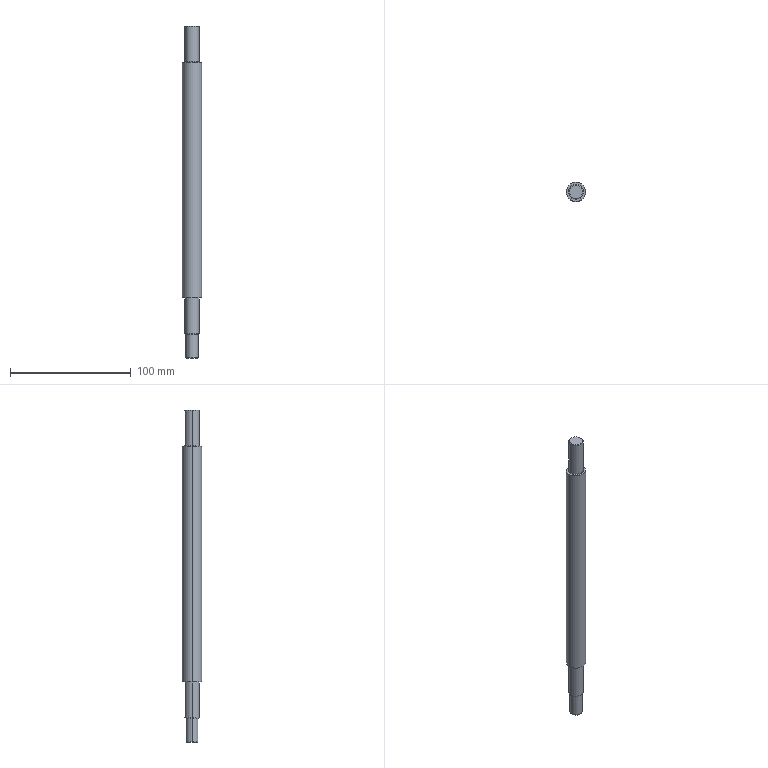Part | STEP file | 0230_001_MTSRK16-275-F30-R12-T30-Q12-S20-E10-BQ15 | 1 solid | 23 faces | box 16 x 16 x 275 mm | volume 47560 mm3 | cylinder 8 | torus 6 | plane 5 | cone 4 | commonest cylinder face diameters 12 x4 10 x2 16 x2
STEP:
#1=CARTESIAN_POINT('',(0.,0.,0.));
#2=DIRECTION('',(0.,0.,1.));
#3=DIRECTION('',(1.,0.,0.));
#4=AXIS2_PLACEMENT_3D('',#1,#2,#3);
#5=CARTESIAN_POINT('',(-4.6,0.,-245.));
#6=VERTEX_POINT('',#5);
#7=CARTESIAN_POINT('',(4.6,0.,-245.));
#8=VERTEX_POINT('',#7);
#9=CARTESIAN_POINT('',(0.,0.,-245.));
#10=DIRECTION('',(0.,0.,-1.));
#11=DIRECTION('',(-1.,0.,0.));
#12=AXIS2_PLACEMENT_3D('',#9,#10,#11);
#13=CIRCLE('',#12,4.6);
#14=CARTESIAN_POINT('',(0.,0.,-245.));
#15=DIRECTION('',(0.,0.,1.));
#16=DIRECTION('',(1.,0.,0.));
#17=AXIS2_PLACEMENT_3D('',#14,#15,#16);
#18=CONICAL_SURFACE('',#17,4.6,0.7854);
#19=CARTESIAN_POINT('',(3.142,0.));
#20=DIRECTION('',(-1.,0.));
#21=VECTOR('',#20,1.);
#22=LINE('',#19,#21);
#23=(GEOMETRIC_REPRESENTATION_CONTEXT(2)PARAMETRIC_REPRESENTATION_CONTEXT()REPRESENTATION_CONTEXT('',''));
#24=DEFINITIONAL_REPRESENTATION('',(#22),#23);
#25=PCURVE('',#18,#24);
#26=CARTESIAN_POINT('',(0.,0.,-245.));
#27=DIRECTION('',(0.,0.,-1.));
#28=DIRECTION('',(-1.,0.,0.));
#29=AXIS2_PLACEMENT_3D('',#26,#27,#28);
#30=PLANE('',#29);
#31=CARTESIAN_POINT('',(0.,0.));
#32=DIRECTION('',(1.,0.));
#33=AXIS2_PLACEMENT_2D('',#31,#32);
#34=CIRCLE('',#33,4.6);
#35=(GEOMETRIC_REPRESENTATION_CONTEXT(2)PARAMETRIC_REPRESENTATION_CONTEXT()REPRESENTATION_CONTEXT('',''));
#36=DEFINITIONAL_REPRESENTATION('',(#34),#35);
#37=PCURVE('',#30,#36);
#38=SURFACE_CURVE('',#13,(#25,#37),.PCURVE_S1.);
#39=EDGE_CURVE('',#6,#8,#38,.T.);
#40=ORIENTED_EDGE('',*,*,#39,.F.);
#41=CARTESIAN_POINT('',(-5.,0.,-244.6));
#42=VERTEX_POINT('',#41);
#43=CARTESIAN_POINT('',(-4.6,0.,-245.));
#44=DIRECTION('',(-0.7071,0.,0.7071));
#45=VECTOR('',#44,1.);
#46=LINE('',#43,#45);
#47=CARTESIAN_POINT('',(3.142,0.));
#48=DIRECTION('',(0.,1.));
#49=VECTOR('',#48,1.);
#50=LINE('',#47,#49);
#51=(GEOMETRIC_REPRESENTATION_CONTEXT(2)PARAMETRIC_REPRESENTATION_CONTEXT()REPRESENTATION_CONTEXT('',''));
#52=DEFINITIONAL_REPRESENTATION('',(#50),#51);
#53=PCURVE('',#18,#52);
#54=CARTESIAN_POINT('',(0.,0.,-245.));
#55=DIRECTION('',(0.,0.,1.));
#56=DIRECTION('',(1.,0.,0.));
#57=AXIS2_PLACEMENT_3D('',#54,#55,#56);
#58=CONICAL_SURFACE('',#57,4.6,0.7854);
#59=CARTESIAN_POINT('',(3.142,0.));
#60=DIRECTION('',(0.,1.));
#61=VECTOR('',#60,1.);
#62=LINE('',#59,#61);
#63=(GEOMETRIC_REPRESENTATION_CONTEXT(2)PARAMETRIC_REPRESENTATION_CONTEXT()REPRESENTATION_CONTEXT('',''));
#64=DEFINITIONAL_REPRESENTATION('',(#62),#63);
#65=PCURVE('',#58,#64);
#66=SURFACE_CURVE('',#46,(#53,#65),.PCURVE_S1.);
#67=EDGE_CURVE('',#6,#42,#66,.T.);
#68=ORIENTED_EDGE('',*,*,#67,.T.);
#69=CARTESIAN_POINT('',(5.,0.,-244.6));
#70=VERTEX_POINT('',#69);
#71=CARTESIAN_POINT('',(0.,0.,-244.6));
#72=DIRECTION('',(0.,0.,1.));
#73=DIRECTION('',(-1.,0.,0.));
#74=AXIS2_PLACEMENT_3D('',#71,#72,#73);
#75=CIRCLE('',#74,5.);
#76=CARTESIAN_POINT('',(-3.142,0.4));
#77=DIRECTION('',(1.,0.));
#78=VECTOR('',#77,1.);
#79=LINE('',#76,#78);
#80=(GEOMETRIC_REPRESENTATION_CONTEXT(2)PARAMETRIC_REPRESENTATION_CONTEXT()REPRESENTATION_CONTEXT('',''));
#81=DEFINITIONAL_REPRESENTATION('',(#79),#80);
#82=PCURVE('',#18,#81);
#83=CARTESIAN_POINT('',(0.,0.,30.));
#84=DIRECTION('',(0.,0.,-1.));
#85=DIRECTION('',(-1.,0.,0.));
#86=AXIS2_PLACEMENT_3D('',#83,#84,#85);
#87=CYLINDRICAL_SURFACE('',#86,5.);
#88=CARTESIAN_POINT('',(6.283,274.6));
#89=DIRECTION('',(-1.,0.));
#90=VECTOR('',#89,1.);
#91=LINE('',#88,#90);
#92=(GEOMETRIC_REPRESENTATION_CONTEXT(2)PARAMETRIC_REPRESENTATION_CONTEXT()REPRESENTATION_CONTEXT('',''));
#93=DEFINITIONAL_REPRESENTATION('',(#91),#92);
#94=PCURVE('',#87,#93);
#95=SURFACE_CURVE('',#75,(#82,#94),.PCURVE_S1.);
#96=EDGE_CURVE('',#70,#42,#95,.T.);
#97=ORIENTED_EDGE('',*,*,#96,.F.);
#98=CARTESIAN_POINT('',(4.6,0.,-245.));
#99=DIRECTION('',(0.7071,0.,0.7071));
#100=VECTOR('',#99,1.);
#101=LINE('',#98,#100);
#102=CARTESIAN_POINT('',(0.,0.));
#103=DIRECTION('',(0.,1.));
#104=VECTOR('',#103,1.);
#105=LINE('',#102,#104);
#106=(GEOMETRIC_REPRESENTATION_CONTEXT(2)PARAMETRIC_REPRESENTATION_CONTEXT()REPRESENTATION_CONTEXT('',''));
#107=DEFINITIONAL_REPRESENTATION('',(#105),#106);
#108=PCURVE('',#18,#107);
#109=CARTESIAN_POINT('',(6.283,0.));
#110=DIRECTION('',(0.,1.));
#111=VECTOR('',#110,1.);
#112=LINE('',#109,#111);
#113=(GEOMETRIC_REPRESENTATION_CONTEXT(2)PARAMETRIC_REPRESENTATION_CONTEXT()REPRESENTATION_CONTEXT('',''));
#114=DEFINITIONAL_REPRESENTATION('',(#112),#113);
#115=PCURVE('',#58,#114);
#116=SURFACE_CURVE('',#101,(#108,#115),.PCURVE_S1.);
#117=EDGE_CURVE('',#8,#70,#116,.T.);
#118=ORIENTED_EDGE('',*,*,#117,.F.);
#119=EDGE_LOOP('',(#40,#68,#97,#118));
#120=FACE_BOUND('',#119,.T.);
#121=ADVANCED_FACE('',(#120),#18,.T.);
#122=CARTESIAN_POINT('',(5.6,0.,30.));
#123=VERTEX_POINT('',#122);
#124=CARTESIAN_POINT('',(-5.6,0.,30.));
#125=VERTEX_POINT('',#124);
#126=CARTESIAN_POINT('',(0.,0.,30.));
#127=DIRECTION('',(0.,0.,1.));
#128=DIRECTION('',(1.,0.,0.));
#129=AXIS2_PLACEMENT_3D('',#126,#127,#128);
#130=CIRCLE('',#129,5.6);
#131=CARTESIAN_POINT('',(0.,0.,29.6));
#132=DIRECTION('',(0.,0.,-1.));
#133=DIRECTION('',(-1.,0.,0.));
#134=AXIS2_PLACEMENT_3D('',#131,#132,#133);
#135=CONICAL_SURFACE('',#134,6.,0.7854);
#136=CARTESIAN_POINT('',(3.142,-0.4));
#137=DIRECTION('',(-1.,0.));
#138=VECTOR('',#137,1.);
#139=LINE('',#136,#138);
#140=(GEOMETRIC_REPRESENTATION_CONTEXT(2)PARAMETRIC_REPRESENTATION_CONTEXT()REPRESENTATION_CONTEXT('',''));
#141=DEFINITIONAL_REPRESENTATION('',(#139),#140);
#142=PCURVE('',#135,#141);
#143=CARTESIAN_POINT('',(6.,0.,30.));
#144=DIRECTION('',(0.,0.,1.));
#145=DIRECTION('',(1.,0.,0.));
#146=AXIS2_PLACEMENT_3D('',#143,#144,#145);
#147=PLANE('',#146);
#148=CARTESIAN_POINT('',(-6.,0.));
#149=DIRECTION('',(1.,0.));
#150=AXIS2_PLACEMENT_2D('',#148,#149);
#151=CIRCLE('',#150,5.6);
#152=(GEOMETRIC_REPRESENTATION_CONTEXT(2)PARAMETRIC_REPRESENTATION_CONTEXT()REPRESENTATION_CONTEXT('',''));
#153=DEFINITIONAL_REPRESENTATION('',(#151),#152);
#154=PCURVE('',#147,#153);
#155=SURFACE_CURVE('',#130,(#142,#154),.PCURVE_S1.);
#156=EDGE_CURVE('',#123,#125,#155,.T.);
#157=ORIENTED_EDGE('',*,*,#156,.F.);
#158=CARTESIAN_POINT('',(6.,0.,29.6));
#159=VERTEX_POINT('',#158);
#160=CARTESIAN_POINT('',(6.,0.,29.6));
#161=DIRECTION('',(0.7071,0.,-0.7071));
#162=VECTOR('',#161,1.);
#163=LINE('',#160,#162);
#164=CARTESIAN_POINT('',(3.142,0.));
#165=DIRECTION('',(0.,1.));
#166=VECTOR('',#165,1.);
#167=LINE('',#164,#166);
#168=(GEOMETRIC_REPRESENTATION_CONTEXT(2)PARAMETRIC_REPRESENTATION_CONTEXT()REPRESENTATION_CONTEXT('',''));
#169=DEFINITIONAL_REPRESENTATION('',(#167),#168);
#170=PCURVE('',#135,#169);
#171=CARTESIAN_POINT('',(0.,0.,29.6));
#172=DIRECTION('',(0.,0.,-1.));
#173=DIRECTION('',(-1.,0.,0.));
#174=AXIS2_PLACEMENT_3D('',#171,#172,#173);
#175=CONICAL_SURFACE('',#174,6.,0.7854);
#176=CARTESIAN_POINT('',(3.142,0.));
#177=DIRECTION('',(0.,1.));
#178=VECTOR('',#177,1.);
#179=LINE('',#176,#178);
#180=(GEOMETRIC_REPRESENTATION_CONTEXT(2)PARAMETRIC_REPRESENTATION_CONTEXT()REPRESENTATION_CONTEXT('',''));
#181=DEFINITIONAL_REPRESENTATION('',(#179),#180);
#182=PCURVE('',#175,#181);
#183=SURFACE_CURVE('',#163,(#170,#182),.PCURVE_S1.);
#184=EDGE_CURVE('',#123,#159,#183,.T.);
#185=ORIENTED_EDGE('',*,*,#184,.T.);
#186=CARTESIAN_POINT('',(-6.,0.,29.6));
#187=VERTEX_POINT('',#186);
#188=CARTESIAN_POINT('',(0.,0.,29.6));
#189=DIRECTION('',(0.,0.,-1.));
#190=DIRECTION('',(1.,0.,0.));
#191=AXIS2_PLACEMENT_3D('',#188,#189,#190);
#192=CIRCLE('',#191,6.);
#193=CARTESIAN_POINT('',(-3.142,0.));
#194=DIRECTION('',(1.,0.));
#195=VECTOR('',#194,1.);
#196=LINE('',#193,#195);
#197=(GEOMETRIC_REPRESENTATION_CONTEXT(2)PARAMETRIC_REPRESENTATION_CONTEXT()REPRESENTATION_CONTEXT('',''));
#198=DEFINITIONAL_REPRESENTATION('',(#196),#197);
#199=PCURVE('',#135,#198);
#200=CARTESIAN_POINT('',(0.,0.,30.));
#201=DIRECTION('',(0.,0.,-1.));
#202=DIRECTION('',(-1.,0.,0.));
#203=AXIS2_PLACEMENT_3D('',#200,#201,#202);
#204=CYLINDRICAL_SURFACE('',#203,6.);
#205=CARTESIAN_POINT('',(-3.142,0.4));
#206=DIRECTION('',(1.,0.));
#207=VECTOR('',#206,1.);
#208=LINE('',#205,#207);
#209=(GEOMETRIC_REPRESENTATION_CONTEXT(2)PARAMETRIC_REPRESENTATION_CONTEXT()REPRESENTATION_CONTEXT('',''));
#210=DEFINITIONAL_REPRESENTATION('',(#208),#209);
#211=PCURVE('',#204,#210);
#212=SURFACE_CURVE('',#192,(#199,#211),.PCURVE_S1.);
#213=EDGE_CURVE('',#187,#159,#212,.T.);
#214=ORIENTED_EDGE('',*,*,#213,.F.);
#215=CARTESIAN_POINT('',(-6.,0.,29.6));
#216=DIRECTION('',(-0.7071,0.,-0.7071));
#217=VECTOR('',#216,1.);
#218=LINE('',#215,#217);
#219=CARTESIAN_POINT('',(0.,0.));
#220=DIRECTION('',(0.,1.));
#221=VECTOR('',#220,1.);
#222=LINE('',#219,#221);
#223=(GEOMETRIC_REPRESENTATION_CONTEXT(2)PARAMETRIC_REPRESENTATION_CONTEXT()REPRESENTATION_CONTEXT('',''));
#224=DEFINITIONAL_REPRESENTATION('',(#222),#223);
#225=PCURVE('',#135,#224);
#226=CARTESIAN_POINT('',(6.283,0.));
#227=DIRECTION('',(0.,1.));
#228=VECTOR('',#227,1.);
#229=LINE('',#226,#228);
#230=(GEOMETRIC_REPRESENTATION_CONTEXT(2)PARAMETRIC_REPRESENTATION_CONTEXT()REPRESENTATION_CONTEXT('',''));
#231=DEFINITIONAL_REPRESENTATION('',(#229),#230);
#232=PCURVE('',#175,#231);
#233=SURFACE_CURVE('',#218,(#225,#232),.PCURVE_S1.);
#234=EDGE_CURVE('',#125,#187,#233,.T.);
#235=ORIENTED_EDGE('',*,*,#234,.F.);
#236=EDGE_LOOP('',(#157,#185,#214,#235));
#237=FACE_BOUND('',#236,.T.);
#238=ADVANCED_FACE('',(#237),#135,.T.);
#239=CARTESIAN_POINT('',(6.,0.,0.3));
#240=VERTEX_POINT('',#239);
#241=CARTESIAN_POINT('',(6.3,0.,0.));
#242=VERTEX_POINT('',#241);
#243=CARTESIAN_POINT('',(6.3,0.,0.3));
#244=DIRECTION('',(0.,-1.,0.));
#245=DIRECTION('',(0.,0.,-1.));
#246=AXIS2_PLACEMENT_3D('',#243,#244,#245);
#247=CIRCLE('',#246,0.3);
#248=CARTESIAN_POINT('',(0.,0.,0.3));
#249=DIRECTION('',(0.,0.,1.));
#250=DIRECTION('',(1.,0.,0.));
#251=AXIS2_PLACEMENT_3D('',#248,#249,#250);
#252=TOROIDAL_SURFACE('',#251,6.3,0.3);
#253=CARTESIAN_POINT('',(6.283,-1.571));
#254=DIRECTION('',(0.,1.));
#255=VECTOR('',#254,1.);
#256=LINE('',#253,#255);
#257=(GEOMETRIC_REPRESENTATION_CONTEXT(2)PARAMETRIC_REPRESENTATION_CONTEXT()REPRESENTATION_CONTEXT('',''));
#258=DEFINITIONAL_REPRESENTATION('',(#256),#257);
#259=PCURVE('',#252,#258);
#260=CARTESIAN_POINT('',(0.,0.,0.3));
#261=DIRECTION('',(0.,0.,1.));
#262=DIRECTION('',(1.,0.,0.));
#263=AXIS2_PLACEMENT_3D('',#260,#261,#262);
#264=TOROIDAL_SURFACE('',#263,6.3,0.3);
#265=CARTESIAN_POINT('',(0.,-1.571));
#266=DIRECTION('',(0.,1.));
#267=VECTOR('',#266,1.);
#268=LINE('',#265,#267);
#269=(GEOMETRIC_REPRESENTATION_CONTEXT(2)PARAMETRIC_REPRESENTATION_CONTEXT()REPRESENTATION_CONTEXT('',''));
#270=DEFINITIONAL_REPRESENTATION('',(#268),#269);
#271=PCURVE('',#264,#270);
#272=SURFACE_CURVE('',#247,(#259,#271),.PCURVE_S1.);
#273=EDGE_CURVE('',#240,#242,#272,.T.);
#274=ORIENTED_EDGE('',*,*,#273,.T.);
#275=CARTESIAN_POINT('',(-6.3,0.,0.));
#276=VERTEX_POINT('',#275);
#277=CARTESIAN_POINT('',(0.,0.,0.));
#278=DIRECTION('',(0.,0.,-1.));
#279=DIRECTION('',(1.,0.,0.));
#280=AXIS2_PLACEMENT_3D('',#277,#278,#279);
#281=CIRCLE('',#280,6.3);
#282=CARTESIAN_POINT('',(6.283,4.712));
#283=DIRECTION('',(-1.,0.));
#284=VECTOR('',#283,1.);
#285=LINE('',#282,#284);
#286=(GEOMETRIC_REPRESENTATION_CONTEXT(2)PARAMETRIC_REPRESENTATION_CONTEXT()REPRESENTATION_CONTEXT('',''));
#287=DEFINITIONAL_REPRESENTATION('',(#285),#286);
#288=PCURVE('',#252,#287);
#289=CARTESIAN_POINT('',(8.,0.,0.));
#290=DIRECTION('',(0.,0.,1.));
#291=DIRECTION('',(1.,0.,0.));
#292=AXIS2_PLACEMENT_3D('',#289,#290,#291);
#293=PLANE('',#292);
#294=CARTESIAN_POINT('',(-1.7,0.));
#295=CARTESIAN_POINT('',(-1.7,-10.912));
#296=CARTESIAN_POINT('',(-11.15,-5.456));
#297=CARTESIAN_POINT('',(-20.6,0.));
#298=CARTESIAN_POINT('',(-11.15,5.456));
#299=CARTESIAN_POINT('',(-1.7,10.912));
#300=CARTESIAN_POINT('',(-1.7,0.));
#301=(BOUNDED_CURVE()B_SPLINE_CURVE(2,(#294,#295,#296,#297,#298,#299,#300),.UNSPECIFIED.,.T.,.F.)B_SPLINE_CURVE_WITH_KNOTS((1,2,2,2,2,1),(-2.094,0.,2.094,4.189,6.283,8.378),.UNSPECIFIED.)CURVE()GEOMETRIC_REPRESENTATION_ITEM()RATIONAL_B_SPLINE_CURVE((1.,0.5,1.,0.5,1.,0.5,1.))REPRESENTATION_ITEM(''));
#302=(GEOMETRIC_REPRESENTATION_CONTEXT(2)PARAMETRIC_REPRESENTATION_CONTEXT()REPRESENTATION_CONTEXT('',''));
#303=DEFINITIONAL_REPRESENTATION('',(#301),#302);
#304=PCURVE('',#293,#303);
#305=SURFACE_CURVE('',#281,(#288,#304),.PCURVE_S1.);
#306=EDGE_CURVE('',#242,#276,#305,.T.);
#307=ORIENTED_EDGE('',*,*,#306,.T.);
#308=CARTESIAN_POINT('',(-6.,0.,0.3));
#309=VERTEX_POINT('',#308);
#310=CARTESIAN_POINT('',(-6.3,0.,0.3));
#311=DIRECTION('',(0.,1.,0.));
#312=DIRECTION('',(-1.,0.,0.));
#313=AXIS2_PLACEMENT_3D('',#310,#311,#312);
#314=CIRCLE('',#313,0.3);
#315=CARTESIAN_POINT('',(3.142,0.));
#316=DIRECTION('',(0.,1.));
#317=VECTOR('',#316,1.);
#318=LINE('',#315,#317);
#319=(GEOMETRIC_REPRESENTATION_CONTEXT(2)PARAMETRIC_REPRESENTATION_CONTEXT()REPRESENTATION_CONTEXT('',''));
#320=DEFINITIONAL_REPRESENTATION('',(#318),#319);
#321=PCURVE('',#252,#320);
#322=CARTESIAN_POINT('',(3.142,0.));
#323=DIRECTION('',(0.,1.));
#324=VECTOR('',#323,1.);
#325=LINE('',#322,#324);
#326=(GEOMETRIC_REPRESENTATION_CONTEXT(2)PARAMETRIC_REPRESENTATION_CONTEXT()REPRESENTATION_CONTEXT('',''));
#327=DEFINITIONAL_REPRESENTATION('',(#325),#326);
#328=PCURVE('',#264,#327);
#329=SURFACE_CURVE('',#314,(#321,#328),.PCURVE_S1.);
#330=EDGE_CURVE('',#309,#276,#329,.T.);
#331=ORIENTED_EDGE('',*,*,#330,.F.);
#332=CARTESIAN_POINT('',(0.,0.,0.3));
#333=DIRECTION('',(0.,0.,1.));
#334=DIRECTION('',(1.,0.,0.));
#335=AXIS2_PLACEMENT_3D('',#332,#333,#334);
#336=CIRCLE('',#335,6.);
#337=CARTESIAN_POINT('',(0.,3.142));
#338=DIRECTION('',(1.,0.));
#339=VECTOR('',#338,1.);
#340=LINE('',#337,#339);
#341=(GEOMETRIC_REPRESENTATION_CONTEXT(2)PARAMETRIC_REPRESENTATION_CONTEXT()REPRESENTATION_CONTEXT('',''));
#342=DEFINITIONAL_REPRESENTATION('',(#340),#341);
#343=PCURVE('',#252,#342);
#344=CARTESIAN_POINT('',(0.,0.,30.));
#345=DIRECTION('',(0.,0.,-1.));
#346=DIRECTION('',(-1.,0.,0.));
#347=AXIS2_PLACEMENT_3D('',#344,#345,#346);
#348=CYLINDRICAL_SURFACE('',#347,6.);
#349=CARTESIAN_POINT('',(9.425,29.7));
#350=DIRECTION('',(-1.,0.));
#351=VECTOR('',#350,1.);
#352=LINE('',#349,#351);
#353=(GEOMETRIC_REPRESENTATION_CONTEXT(2)PARAMETRIC_REPRESENTATION_CONTEXT()REPRESENTATION_CONTEXT('',''));
#354=DEFINITIONAL_REPRESENTATION('',(#352),#353);
#355=PCURVE('',#348,#354);
#356=SURFACE_CURVE('',#336,(#343,#355),.PCURVE_S1.);
#357=EDGE_CURVE('',#309,#240,#356,.T.);
#358=ORIENTED_EDGE('',*,*,#357,.T.);
#359=EDGE_LOOP('',(#274,#307,#331,#358));
#360=FACE_BOUND('',#359,.F.);
#361=ADVANCED_FACE('',(#360),#252,.F.);
#362=CARTESIAN_POINT('',(-6.,0.,-195.3));
#363=VERTEX_POINT('',#362);
#364=CARTESIAN_POINT('',(-6.3,0.,-195.));
#365=VERTEX_POINT('',#364);
#366=CARTESIAN_POINT('',(-6.3,0.,-195.3));
#367=DIRECTION('',(0.,-1.,0.));
#368=DIRECTION('',(0.,0.,-1.));
#369=AXIS2_PLACEMENT_3D('',#366,#367,#368);
#370=CIRCLE('',#369,0.3);
#371=CARTESIAN_POINT('',(0.,0.,-195.3));
#372=DIRECTION('',(0.,0.,-1.));
#373=DIRECTION('',(-1.,0.,0.));
#374=AXIS2_PLACEMENT_3D('',#371,#372,#373);
#375=TOROIDAL_SURFACE('',#374,6.3,0.3);
#376=CARTESIAN_POINT('',(6.283,1.571));
#377=DIRECTION('',(0.,1.));
#378=VECTOR('',#377,1.);
#379=LINE('',#376,#378);
#380=(GEOMETRIC_REPRESENTATION_CONTEXT(2)PARAMETRIC_REPRESENTATION_CONTEXT()REPRESENTATION_CONTEXT('',''));
#381=DEFINITIONAL_REPRESENTATION('',(#379),#380);
#382=PCURVE('',#375,#381);
#383=CARTESIAN_POINT('',(0.,0.,-195.3));
#384=DIRECTION('',(0.,0.,-1.));
#385=DIRECTION('',(-1.,0.,0.));
#386=AXIS2_PLACEMENT_3D('',#383,#384,#385);
#387=TOROIDAL_SURFACE('',#386,6.3,0.3);
#388=CARTESIAN_POINT('',(0.,1.571));
#389=DIRECTION('',(0.,1.));
#390=VECTOR('',#389,1.);
#391=LINE('',#388,#390);
#392=(GEOMETRIC_REPRESENTATION_CONTEXT(2)PARAMETRIC_REPRESENTATION_CONTEXT()REPRESENTATION_CONTEXT('',''));
#393=DEFINITIONAL_REPRESENTATION('',(#391),#392);
#394=PCURVE('',#387,#393);
#395=SURFACE_CURVE('',#370,(#382,#394),.PCURVE_S1.);
#396=EDGE_CURVE('',#363,#365,#395,.T.);
#397=ORIENTED_EDGE('',*,*,#396,.T.);
#398=CARTESIAN_POINT('',(6.3,0.,-195.));
#399=VERTEX_POINT('',#398);
#400=CARTESIAN_POINT('',(0.,0.,-195.));
#401=DIRECTION('',(0.,0.,1.));
#402=DIRECTION('',(-1.,0.,0.));
#403=AXIS2_PLACEMENT_3D('',#400,#401,#402);
#404=CIRCLE('',#403,6.3);
#405=CARTESIAN_POINT('',(6.283,4.712));
#406=DIRECTION('',(-1.,0.));
#407=VECTOR('',#406,1.);
#408=LINE('',#405,#407);
#409=(GEOMETRIC_REPRESENTATION_CONTEXT(2)PARAMETRIC_REPRESENTATION_CONTEXT()REPRESENTATION_CONTEXT('',''));
#410=DEFINITIONAL_REPRESENTATION('',(#408),#409);
#411=PCURVE('',#375,#410);
#412=CARTESIAN_POINT('',(6.,0.,-195.));
#413=DIRECTION('',(0.,0.,-1.));
#414=DIRECTION('',(-1.,0.,0.));
#415=AXIS2_PLACEMENT_3D('',#412,#413,#414);
#416=PLANE('',#415);
#417=CARTESIAN_POINT('',(12.3,0.));
#418=CARTESIAN_POINT('',(12.3,-10.912));
#419=CARTESIAN_POINT('',(2.85,-5.456));
#420=CARTESIAN_POINT('',(-6.6,0.));
#421=CARTESIAN_POINT('',(2.85,5.456));
#422=CARTESIAN_POINT('',(12.3,10.912));
#423=CARTESIAN_POINT('',(12.3,0.));
#424=(BOUNDED_CURVE()B_SPLINE_CURVE(2,(#417,#418,#419,#420,#421,#422,#423),.UNSPECIFIED.,.T.,.F.)B_SPLINE_CURVE_WITH_KNOTS((1,2,2,2,2,1),(-2.094,0.,2.094,4.189,6.283,8.378),.UNSPECIFIED.)CURVE()GEOMETRIC_REPRESENTATION_ITEM()RATIONAL_B_SPLINE_CURVE((1.,0.5,1.,0.5,1.,0.5,1.))REPRESENTATION_ITEM(''));
#425=(GEOMETRIC_REPRESENTATION_CONTEXT(2)PARAMETRIC_REPRESENTATION_CONTEXT()REPRESENTATION_CONTEXT('',''));
#426=DEFINITIONAL_REPRESENTATION('',(#424),#425);
#427=PCURVE('',#416,#426);
#428=SURFACE_CURVE('',#404,(#411,#427),.PCURVE_S1.);
#429=EDGE_CURVE('',#365,#399,#428,.T.);
#430=ORIENTED_EDGE('',*,*,#429,.T.);
#431=CARTESIAN_POINT('',(6.,0.,-195.3));
#432=VERTEX_POINT('',#431);
#433=CARTESIAN_POINT('',(6.3,0.,-195.3));
#434=DIRECTION('',(0.,1.,0.));
#435=DIRECTION('',(-1.,0.,0.));
#436=AXIS2_PLACEMENT_3D('',#433,#434,#435);
#437=CIRCLE('',#436,0.3);
#438=CARTESIAN_POINT('',(3.142,3.142));
#439=DIRECTION('',(0.,1.));
#440=VECTOR('',#439,1.);
#441=LINE('',#438,#440);
#442=(GEOMETRIC_REPRESENTATION_CONTEXT(2)PARAMETRIC_REPRESENTATION_CONTEXT()REPRESENTATION_CONTEXT('',''));
#443=DEFINITIONAL_REPRESENTATION('',(#441),#442);
#444=PCURVE('',#375,#443);
#445=CARTESIAN_POINT('',(3.142,3.142));
#446=DIRECTION('',(0.,1.));
#447=VECTOR('',#446,1.);
#448=LINE('',#445,#447);
#449=(GEOMETRIC_REPRESENTATION_CONTEXT(2)PARAMETRIC_REPRESENTATION_CONTEXT()REPRESENTATION_CONTEXT('',''));
#450=DEFINITIONAL_REPRESENTATION('',(#448),#449);
#451=PCURVE('',#387,#450);
#452=SURFACE_CURVE('',#437,(#444,#451),.PCURVE_S1.);
#453=EDGE_CURVE('',#432,#399,#452,.T.);
#454=ORIENTED_EDGE('',*,*,#453,.F.);
#455=CARTESIAN_POINT('',(0.,0.,-195.3));
#456=DIRECTION('',(0.,0.,-1.));
#457=DIRECTION('',(-1.,0.,0.));
#458=AXIS2_PLACEMENT_3D('',#455,#456,#457);
#459=CIRCLE('',#458,6.);
#460=CARTESIAN_POINT('',(0.,3.142));
#461=DIRECTION('',(1.,0.));
#462=VECTOR('',#461,1.);
#463=LINE('',#460,#462);
#464=(GEOMETRIC_REPRESENTATION_CONTEXT(2)PARAMETRIC_REPRESENTATION_CONTEXT()REPRESENTATION_CONTEXT('',''));
#465=DEFINITIONAL_REPRESENTATION('',(#463),#464);
#466=PCURVE('',#375,#465);
#467=CARTESIAN_POINT('',(0.,0.,30.));
#468=DIRECTION('',(0.,0.,-1.));
#469=DIRECTION('',(-1.,0.,0.));
#470=AXIS2_PLACEMENT_3D('',#467,#468,#469);
#471=CYLINDRICAL_SURFACE('',#470,6.);
#472=CARTESIAN_POINT('',(0.,225.3));
#473=DIRECTION('',(1.,0.));
#474=VECTOR('',#473,1.);
#475=LINE('',#472,#474);
#476=(GEOMETRIC_REPRESENTATION_CONTEXT(2)PARAMETRIC_REPRESENTATION_CONTEXT()REPRESENTATION_CONTEXT('',''));
#477=DEFINITIONAL_REPRESENTATION('',(#475),#476);
#478=PCURVE('',#471,#477);
#479=SURFACE_CURVE('',#459,(#466,#478),.PCURVE_S1.);
#480=EDGE_CURVE('',#432,#363,#479,.T.);
#481=ORIENTED_EDGE('',*,*,#480,.T.);
#482=EDGE_LOOP('',(#397,#430,#454,#481));
#483=FACE_BOUND('',#482,.F.);
#484=ADVANCED_FACE('',(#483),#375,.F.);
#485=CARTESIAN_POINT('',(-5.,0.,-225.3));
#486=VERTEX_POINT('',#485);
#487=CARTESIAN_POINT('',(-5.3,0.,-225.));
#488=VERTEX_POINT('',#487);
#489=CARTESIAN_POINT('',(-5.3,0.,-225.3));
#490=DIRECTION('',(0.,-1.,0.));
#491=DIRECTION('',(0.,0.,-1.));
#492=AXIS2_PLACEMENT_3D('',#489,#490,#491);
#493=CIRCLE('',#492,0.3);
#494=CARTESIAN_POINT('',(0.,0.,-225.3));
#495=DIRECTION('',(0.,0.,-1.));
#496=DIRECTION('',(-1.,0.,0.));
#497=AXIS2_PLACEMENT_3D('',#494,#495,#496);
#498=TOROIDAL_SURFACE('',#497,5.3,0.3);
#499=CARTESIAN_POINT('',(6.283,1.571));
#500=DIRECTION('',(0.,1.));
#501=VECTOR('',#500,1.);
#502=LINE('',#499,#501);
#503=(GEOMETRIC_REPRESENTATION_CONTEXT(2)PARAMETRIC_REPRESENTATION_CONTEXT()REPRESENTATION_CONTEXT('',''));
#504=DEFINITIONAL_REPRESENTATION('',(#502),#503);
#505=PCURVE('',#498,#504);
#506=CARTESIAN_POINT('',(0.,0.,-225.3));
#507=DIRECTION('',(0.,0.,-1.));
#508=DIRECTION('',(-1.,0.,0.));
#509=AXIS2_PLACEMENT_3D('',#506,#507,#508);
#510=TOROIDAL_SURFACE('',#509,5.3,0.3);
#511=CARTESIAN_POINT('',(0.,1.571));
#512=DIRECTION('',(0.,1.));
#513=VECTOR('',#512,1.);
#514=LINE('',#511,#513);
#515=(GEOMETRIC_REPRESENTATION_CONTEXT(2)PARAMETRIC_REPRESENTATION_CONTEXT()REPRESENTATION_CONTEXT('',''));
#516=DEFINITIONAL_REPRESENTATION('',(#514),#515);
#517=PCURVE('',#510,#516);
#518=SURFACE_CURVE('',#493,(#505,#517),.PCURVE_S1.);
#519=EDGE_CURVE('',#486,#488,#518,.T.);
#520=ORIENTED_EDGE('',*,*,#519,.T.);
#521=CARTESIAN_POINT('',(5.3,0.,-225.));
#522=VERTEX_POINT('',#521);
#523=CARTESIAN_POINT('',(0.,0.,-225.));
#524=DIRECTION('',(0.,0.,1.));
#525=DIRECTION('',(-1.,0.,0.));
#526=AXIS2_PLACEMENT_3D('',#523,#524,#525);
#527=CIRCLE('',#526,5.3);
#528=CARTESIAN_POINT('',(6.283,4.712));
#529=DIRECTION('',(-1.,0.));
#530=VECTOR('',#529,1.);
#531=LINE('',#528,#530);
#532=(GEOMETRIC_REPRESENTATION_CONTEXT(2)PARAMETRIC_REPRESENTATION_CONTEXT()REPRESENTATION_CONTEXT('',''));
#533=DEFINITIONAL_REPRESENTATION('',(#531),#532);
#534=PCURVE('',#498,#533);
#535=CARTESIAN_POINT('',(5.,0.,-225.));
#536=DIRECTION('',(0.,0.,-1.));
#537=DIRECTION('',(-1.,0.,0.));
#538=AXIS2_PLACEMENT_3D('',#535,#536,#537);
#539=PLANE('',#538);
#540=CARTESIAN_POINT('',(10.3,0.));
#541=CARTESIAN_POINT('',(10.3,-9.18));
#542=CARTESIAN_POINT('',(2.35,-4.59));
#543=CARTESIAN_POINT('',(-5.6,0.));
#544=CARTESIAN_POINT('',(2.35,4.59));
#545=CARTESIAN_POINT('',(10.3,9.18));
#546=CARTESIAN_POINT('',(10.3,0.));
#547=(BOUNDED_CURVE()B_SPLINE_CURVE(2,(#540,#541,#542,#543,#544,#545,#546),.UNSPECIFIED.,.T.,.F.)B_SPLINE_CURVE_WITH_KNOTS((1,2,2,2,2,1),(-2.094,0.,2.094,4.189,6.283,8.378),.UNSPECIFIED.)CURVE()GEOMETRIC_REPRESENTATION_ITEM()RATIONAL_B_SPLINE_CURVE((1.,0.5,1.,0.5,1.,0.5,1.))REPRESENTATION_ITEM(''));
#548=(GEOMETRIC_REPRESENTATION_CONTEXT(2)PARAMETRIC_REPRESENTATION_CONTEXT()REPRESENTATION_CONTEXT('',''));
#549=DEFINITIONAL_REPRESENTATION('',(#547),#548);
#550=PCURVE('',#539,#549);
#551=SURFACE_CURVE('',#527,(#534,#550),.PCURVE_S1.);
#552=EDGE_CURVE('',#488,#522,#551,.T.);
#553=ORIENTED_EDGE('',*,*,#552,.T.);
#554=CARTESIAN_POINT('',(5.,0.,-225.3));
#555=VERTEX_POINT('',#554);
#556=CARTESIAN_POINT('',(5.3,0.,-225.3));
#557=DIRECTION('',(0.,1.,0.));
#558=DIRECTION('',(-1.,0.,0.));
#559=AXIS2_PLACEMENT_3D('',#556,#557,#558);
#560=CIRCLE('',#559,0.3);
#561=CARTESIAN_POINT('',(3.142,3.142));
#562=DIRECTION('',(0.,1.));
#563=VECTOR('',#562,1.);
#564=LINE('',#561,#563);
#565=(GEOMETRIC_REPRESENTATION_CONTEXT(2)PARAMETRIC_REPRESENTATION_CONTEXT()REPRESENTATION_CONTEXT('',''));
#566=DEFINITIONAL_REPRESENTATION('',(#564),#565);
#567=PCURVE('',#498,#566);
#568=CARTESIAN_POINT('',(3.142,3.142));
#569=DIRECTION('',(0.,1.));
#570=VECTOR('',#569,1.);
#571=LINE('',#568,#570);
#572=(GEOMETRIC_REPRESENTATION_CONTEXT(2)PARAMETRIC_REPRESENTATION_CONTEXT()REPRESENTATION_CONTEXT('',''));
#573=DEFINITIONAL_REPRESENTATION('',(#571),#572);
#574=PCURVE('',#510,#573);
#575=SURFACE_CURVE('',#560,(#567,#574),.PCURVE_S1.);
#576=EDGE_CURVE('',#555,#522,#575,.T.);
#577=ORIENTED_EDGE('',*,*,#576,.F.);
#578=CARTESIAN_POINT('',(0.,0.,-225.3));
#579=DIRECTION('',(0.,0.,-1.));
#580=DIRECTION('',(-1.,0.,0.));
#581=AXIS2_PLACEMENT_3D('',#578,#579,#580);
#582=CIRCLE('',#581,5.);
#583=CARTESIAN_POINT('',(0.,3.142));
#584=DIRECTION('',(1.,0.));
#585=VECTOR('',#584,1.);
#586=LINE('',#583,#585);
#587=(GEOMETRIC_REPRESENTATION_CONTEXT(2)PARAMETRIC_REPRESENTATION_CONTEXT()REPRESENTATION_CONTEXT('',''));
#588=DEFINITIONAL_REPRESENTATION('',(#586),#587);
#589=PCURVE('',#498,#588);
#590=CARTESIAN_POINT('',(0.,0.,30.));
#591=DIRECTION('',(0.,0.,-1.));
#592=DIRECTION('',(-1.,0.,0.));
#593=AXIS2_PLACEMENT_3D('',#590,#591,#592);
#594=CYLINDRICAL_SURFACE('',#593,5.);
#595=CARTESIAN_POINT('',(0.,255.3));
#596=DIRECTION('',(1.,0.));
#597=VECTOR('',#596,1.);
#598=LINE('',#595,#597);
#599=(GEOMETRIC_REPRESENTATION_CONTEXT(2)PARAMETRIC_REPRESENTATION_CONTEXT()REPRESENTATION_CONTEXT('',''));
#600=DEFINITIONAL_REPRESENTATION('',(#598),#599);
#601=PCURVE('',#594,#600);
#602=SURFACE_CURVE('',#582,(#589,#601),.PCURVE_S1.);
#603=EDGE_CURVE('',#555,#486,#602,.T.);
#604=ORIENTED_EDGE('',*,*,#603,.T.);
#605=EDGE_LOOP('',(#520,#553,#577,#604));
#606=FACE_BOUND('',#605,.F.);
#607=ADVANCED_FACE('',(#606),#498,.F.);
#608=CARTESIAN_POINT('',(-8.,0.,0.));
#609=VERTEX_POINT('',#608);
#610=CARTESIAN_POINT('',(8.,0.,0.));
#611=VERTEX_POINT('',#610);
#612=CARTESIAN_POINT('',(0.,0.,0.));
#613=DIRECTION('',(0.,0.,-1.));
#614=DIRECTION('',(-1.,0.,0.));
#615=AXIS2_PLACEMENT_3D('',#612,#613,#614);
#616=CIRCLE('',#615,8.);
#617=CARTESIAN_POINT('',(0.,0.,30.));
#618=DIRECTION('',(0.,0.,-1.));
#619=DIRECTION('',(-1.,0.,0.));
#620=AXIS2_PLACEMENT_3D('',#617,#618,#619);
#621=CYLINDRICAL_SURFACE('',#620,8.);
#622=CARTESIAN_POINT('',(0.,30.));
#623=DIRECTION('',(1.,0.));
#624=VECTOR('',#623,1.);
#625=LINE('',#622,#624);
#626=(GEOMETRIC_REPRESENTATION_CONTEXT(2)PARAMETRIC_REPRESENTATION_CONTEXT()REPRESENTATION_CONTEXT('',''));
#627=DEFINITIONAL_REPRESENTATION('',(#625),#626);
#628=PCURVE('',#621,#627);
#629=CARTESIAN_POINT('',(-16.,0.));
#630=CARTESIAN_POINT('',(-16.,13.856));
#631=CARTESIAN_POINT('',(-4.,6.928));
#632=CARTESIAN_POINT('',(8.,0.));
#633=CARTESIAN_POINT('',(-4.,-6.928));
#634=CARTESIAN_POINT('',(-16.,-13.856));
#635=CARTESIAN_POINT('',(-16.,0.));
#636=(BOUNDED_CURVE()B_SPLINE_CURVE(2,(#629,#630,#631,#632,#633,#634,#635),.UNSPECIFIED.,.T.,.F.)B_SPLINE_CURVE_WITH_KNOTS((1,2,2,2,2,1),(-2.094,0.,2.094,4.189,6.283,8.378),.UNSPECIFIED.)CURVE()GEOMETRIC_REPRESENTATION_ITEM()RATIONAL_B_SPLINE_CURVE((1.,0.5,1.,0.5,1.,0.5,1.))REPRESENTATION_ITEM(''));
#637=(GEOMETRIC_REPRESENTATION_CONTEXT(2)PARAMETRIC_REPRESENTATION_CONTEXT()REPRESENTATION_CONTEXT('',''));
#638=DEFINITIONAL_REPRESENTATION('',(#636),#637);
#639=PCURVE('',#293,#638);
#640=SURFACE_CURVE('',#616,(#628,#639),.PCURVE_S1.);
#641=EDGE_CURVE('',#609,#611,#640,.T.);
#642=ORIENTED_EDGE('',*,*,#641,.T.);
#643=CARTESIAN_POINT('',(8.,0.,-195.));
#644=VERTEX_POINT('',#643);
#645=CARTESIAN_POINT('',(8.,0.,30.));
#646=DIRECTION('',(0.,0.,-1.));
#647=VECTOR('',#646,1.);
#648=LINE('',#645,#647);
#649=CARTESIAN_POINT('',(3.142,0.));
#650=DIRECTION('',(0.,1.));
#651=VECTOR('',#650,1.);
#652=LINE('',#649,#651);
#653=(GEOMETRIC_REPRESENTATION_CONTEXT(2)PARAMETRIC_REPRESENTATION_CONTEXT()REPRESENTATION_CONTEXT('',''));
#654=DEFINITIONAL_REPRESENTATION('',(#652),#653);
#655=PCURVE('',#621,#654);
#656=CARTESIAN_POINT('',(0.,0.,30.));
#657=DIRECTION('',(0.,0.,-1.));
#658=DIRECTION('',(-1.,0.,0.));
#659=AXIS2_PLACEMENT_3D('',#656,#657,#658);
#660=CYLINDRICAL_SURFACE('',#659,8.);
#661=CARTESIAN_POINT('',(3.142,0.));
#662=DIRECTION('',(0.,1.));
#663=VECTOR('',#662,1.);
#664=LINE('',#661,#663);
#665=(GEOMETRIC_REPRESENTATION_CONTEXT(2)PARAMETRIC_REPRESENTATION_CONTEXT()REPRESENTATION_CONTEXT('',''));
#666=DEFINITIONAL_REPRESENTATION('',(#664),#665);
#667=PCURVE('',#660,#666);
#668=SURFACE_CURVE('',#648,(#655,#667),.PCURVE_S1.);
#669=EDGE_CURVE('',#611,#644,#668,.T.);
#670=ORIENTED_EDGE('',*,*,#669,.T.);
#671=CARTESIAN_POINT('',(-8.,0.,-195.));
#672=VERTEX_POINT('',#671);
#673=CARTESIAN_POINT('',(0.,0.,-195.));
#674=DIRECTION('',(0.,0.,-1.));
#675=DIRECTION('',(-1.,0.,0.));
#676=AXIS2_PLACEMENT_3D('',#673,#674,#675);
#677=CIRCLE('',#676,8.);
#678=CARTESIAN_POINT('',(0.,225.));
#679=DIRECTION('',(1.,0.));
#680=VECTOR('',#679,1.);
#681=LINE('',#678,#680);
#682=(GEOMETRIC_REPRESENTATION_CONTEXT(2)PARAMETRIC_REPRESENTATION_CONTEXT()REPRESENTATION_CONTEXT('',''));
#683=DEFINITIONAL_REPRESENTATION('',(#681),#682);
#684=PCURVE('',#621,#683);
#685=CARTESIAN_POINT('',(6.,0.));
#686=DIRECTION('',(1.,0.));
#687=AXIS2_PLACEMENT_2D('',#685,#686);
#688=CIRCLE('',#687,8.);
#689=(GEOMETRIC_REPRESENTATION_CONTEXT(2)PARAMETRIC_REPRESENTATION_CONTEXT()REPRESENTATION_CONTEXT('',''));
#690=DEFINITIONAL_REPRESENTATION('',(#688),#689);
#691=PCURVE('',#416,#690);
#692=SURFACE_CURVE('',#677,(#684,#691),.PCURVE_S1.);
#693=EDGE_CURVE('',#672,#644,#692,.T.);
#694=ORIENTED_EDGE('',*,*,#693,.F.);
#695=CARTESIAN_POINT('',(-8.,0.,30.));
#696=DIRECTION('',(0.,0.,-1.));
#697=VECTOR('',#696,1.);
#698=LINE('',#695,#697);
#699=CARTESIAN_POINT('',(0.,0.));
#700=DIRECTION('',(0.,1.));
#701=VECTOR('',#700,1.);
#702=LINE('',#699,#701);
#703=(GEOMETRIC_REPRESENTATION_CONTEXT(2)PARAMETRIC_REPRESENTATION_CONTEXT()REPRESENTATION_CONTEXT('',''));
#704=DEFINITIONAL_REPRESENTATION('',(#702),#703);
#705=PCURVE('',#621,#704);
#706=CARTESIAN_POINT('',(6.283,0.));
#707=DIRECTION('',(0.,1.));
#708=VECTOR('',#707,1.);
#709=LINE('',#706,#708);
#710=(GEOMETRIC_REPRESENTATION_CONTEXT(2)PARAMETRIC_REPRESENTATION_CONTEXT()REPRESENTATION_CONTEXT('',''));
#711=DEFINITIONAL_REPRESENTATION('',(#709),#710);
#712=PCURVE('',#660,#711);
#713=SURFACE_CURVE('',#698,(#705,#712),.PCURVE_S1.);
#714=EDGE_CURVE('',#609,#672,#713,.T.);
#715=ORIENTED_EDGE('',*,*,#714,.F.);
#716=EDGE_LOOP('',(#642,#670,#694,#715));
#717=FACE_BOUND('',#716,.T.);
#718=ADVANCED_FACE('',(#717),#621,.T.);
#719=CARTESIAN_POINT('',(0.,0.,-195.3));
#720=DIRECTION('',(0.,0.,-1.));
#721=DIRECTION('',(-1.,0.,0.));
#722=AXIS2_PLACEMENT_3D('',#719,#720,#721);
#723=CIRCLE('',#722,6.);
#724=CARTESIAN_POINT('',(0.,0.,30.));
#725=DIRECTION('',(0.,0.,-1.));
#726=DIRECTION('',(-1.,0.,0.));
#727=AXIS2_PLACEMENT_3D('',#724,#725,#726);
#728=CYLINDRICAL_SURFACE('',#727,6.);
#729=CARTESIAN_POINT('',(0.,225.3));
#730=DIRECTION('',(1.,0.));
#731=VECTOR('',#730,1.);
#732=LINE('',#729,#731);
#733=(GEOMETRIC_REPRESENTATION_CONTEXT(2)PARAMETRIC_REPRESENTATION_CONTEXT()REPRESENTATION_CONTEXT('',''));
#734=DEFINITIONAL_REPRESENTATION('',(#732),#733);
#735=PCURVE('',#728,#734);
#736=CARTESIAN_POINT('',(0.,3.142));
#737=DIRECTION('',(1.,0.));
#738=VECTOR('',#737,1.);
#739=LINE('',#736,#738);
#740=(GEOMETRIC_REPRESENTATION_CONTEXT(2)PARAMETRIC_REPRESENTATION_CONTEXT()REPRESENTATION_CONTEXT('',''));
#741=DEFINITIONAL_REPRESENTATION('',(#739),#740);
#742=PCURVE('',#387,#741);
#743=SURFACE_CURVE('',#723,(#735,#742),.PCURVE_S1.);
#744=EDGE_CURVE('',#363,#432,#743,.T.);
#745=ORIENTED_EDGE('',*,*,#744,.T.);
#746=CARTESIAN_POINT('',(6.,0.,-225.));
#747=VERTEX_POINT('',#746);
#748=CARTESIAN_POINT('',(6.,0.,30.));
#749=DIRECTION('',(0.,0.,-1.));
#750=VECTOR('',#749,1.);
#751=LINE('',#748,#750);
#752=CARTESIAN_POINT('',(3.142,0.));
#753=DIRECTION('',(0.,1.));
#754=VECTOR('',#753,1.);
#755=LINE('',#752,#754);
#756=(GEOMETRIC_REPRESENTATION_CONTEXT(2)PARAMETRIC_REPRESENTATION_CONTEXT()REPRESENTATION_CONTEXT('',''));
#757=DEFINITIONAL_REPRESENTATION('',(#755),#756);
#758=PCURVE('',#728,#757);
#759=CARTESIAN_POINT('',(3.142,0.));
#760=DIRECTION('',(0.,1.));
#761=VECTOR('',#760,1.);
#762=LINE('',#759,#761);
#763=(GEOMETRIC_REPRESENTATION_CONTEXT(2)PARAMETRIC_REPRESENTATION_CONTEXT()REPRESENTATION_CONTEXT('',''));
#764=DEFINITIONAL_REPRESENTATION('',(#762),#763);
#765=PCURVE('',#471,#764);
#766=SURFACE_CURVE('',#751,(#758,#765),.PCURVE_S1.);
#767=EDGE_CURVE('',#432,#747,#766,.T.);
#768=ORIENTED_EDGE('',*,*,#767,.T.);
#769=CARTESIAN_POINT('',(-6.,0.,-225.));
#770=VERTEX_POINT('',#769);
#771=CARTESIAN_POINT('',(0.,0.,-225.));
#772=DIRECTION('',(0.,0.,-1.));
#773=DIRECTION('',(-1.,0.,0.));
#774=AXIS2_PLACEMENT_3D('',#771,#772,#773);
#775=CIRCLE('',#774,6.);
#776=CARTESIAN_POINT('',(0.,255.));
#777=DIRECTION('',(1.,0.));
#778=VECTOR('',#777,1.);
#779=LINE('',#776,#778);
#780=(GEOMETRIC_REPRESENTATION_CONTEXT(2)PARAMETRIC_REPRESENTATION_CONTEXT()REPRESENTATION_CONTEXT('',''));
#781=DEFINITIONAL_REPRESENTATION('',(#779),#780);
#782=PCURVE('',#728,#781);
#783=CARTESIAN_POINT('',(5.,0.));
#784=DIRECTION('',(1.,0.));
#785=AXIS2_PLACEMENT_2D('',#783,#784);
#786=CIRCLE('',#785,6.);
#787=(GEOMETRIC_REPRESENTATION_CONTEXT(2)PARAMETRIC_REPRESENTATION_CONTEXT()REPRESENTATION_CONTEXT('',''));
#788=DEFINITIONAL_REPRESENTATION('',(#786),#787);
#789=PCURVE('',#539,#788);
#790=SURFACE_CURVE('',#775,(#782,#789),.PCURVE_S1.);
#791=EDGE_CURVE('',#770,#747,#790,.T.);
#792=ORIENTED_EDGE('',*,*,#791,.F.);
#793=CARTESIAN_POINT('',(-6.,0.,30.));
#794=DIRECTION('',(0.,0.,-1.));
#795=VECTOR('',#794,1.);
#796=LINE('',#793,#795);
#797=CARTESIAN_POINT('',(0.,0.));
#798=DIRECTION('',(0.,1.));
#799=VECTOR('',#798,1.);
#800=LINE('',#797,#799);
#801=(GEOMETRIC_REPRESENTATION_CONTEXT(2)PARAMETRIC_REPRESENTATION_CONTEXT()REPRESENTATION_CONTEXT('',''));
#802=DEFINITIONAL_REPRESENTATION('',(#800),#801);
#803=PCURVE('',#728,#802);
#804=CARTESIAN_POINT('',(6.283,0.));
#805=DIRECTION('',(0.,1.));
#806=VECTOR('',#805,1.);
#807=LINE('',#804,#806);
#808=(GEOMETRIC_REPRESENTATION_CONTEXT(2)PARAMETRIC_REPRESENTATION_CONTEXT()REPRESENTATION_CONTEXT('',''));
#809=DEFINITIONAL_REPRESENTATION('',(#807),#808);
#810=PCURVE('',#471,#809);
#811=SURFACE_CURVE('',#796,(#803,#810),.PCURVE_S1.);
#812=EDGE_CURVE('',#363,#770,#811,.T.);
#813=ORIENTED_EDGE('',*,*,#812,.F.);
#814=EDGE_LOOP('',(#745,#768,#792,#813));
#815=FACE_BOUND('',#814,.T.);
#816=ADVANCED_FACE('',(#815),#728,.T.);
#817=CARTESIAN_POINT('',(0.,0.,-225.3));
#818=DIRECTION('',(0.,0.,-1.));
#819=DIRECTION('',(-1.,0.,0.));
#820=AXIS2_PLACEMENT_3D('',#817,#818,#819);
#821=CIRCLE('',#820,5.);
#822=CARTESIAN_POINT('',(0.,255.3));
#823=DIRECTION('',(1.,0.));
#824=VECTOR('',#823,1.);
#825=LINE('',#822,#824);
#826=(GEOMETRIC_REPRESENTATION_CONTEXT(2)PARAMETRIC_REPRESENTATION_CONTEXT()REPRESENTATION_CONTEXT('',''));
#827=DEFINITIONAL_REPRESENTATION('',(#825),#826);
#828=PCURVE('',#87,#827);
#829=CARTESIAN_POINT('',(0.,3.142));
#830=DIRECTION('',(1.,0.));
#831=VECTOR('',#830,1.);
#832=LINE('',#829,#831);
#833=(GEOMETRIC_REPRESENTATION_CONTEXT(2)PARAMETRIC_REPRESENTATION_CONTEXT()REPRESENTATION_CONTEXT('',''));
#834=DEFINITIONAL_REPRESENTATION('',(#832),#833);
#835=PCURVE('',#510,#834);
#836=SURFACE_CURVE('',#821,(#828,#835),.PCURVE_S1.);
#837=EDGE_CURVE('',#486,#555,#836,.T.);
#838=ORIENTED_EDGE('',*,*,#837,.T.);
#839=CARTESIAN_POINT('',(5.,0.,30.));
#840=DIRECTION('',(0.,0.,-1.));
#841=VECTOR('',#840,1.);
#842=LINE('',#839,#841);
#843=CARTESIAN_POINT('',(3.142,0.));
#844=DIRECTION('',(0.,1.));
#845=VECTOR('',#844,1.);
#846=LINE('',#843,#845);
#847=(GEOMETRIC_REPRESENTATION_CONTEXT(2)PARAMETRIC_REPRESENTATION_CONTEXT()REPRESENTATION_CONTEXT('',''));
#848=DEFINITIONAL_REPRESENTATION('',(#846),#847);
#849=PCURVE('',#87,#848);
#850=CARTESIAN_POINT('',(3.142,0.));
#851=DIRECTION('',(0.,1.));
#852=VECTOR('',#851,1.);
#853=LINE('',#850,#852);
#854=(GEOMETRIC_REPRESENTATION_CONTEXT(2)PARAMETRIC_REPRESENTATION_CONTEXT()REPRESENTATION_CONTEXT('',''));
#855=DEFINITIONAL_REPRESENTATION('',(#853),#854);
#856=PCURVE('',#594,#855);
#857=SURFACE_CURVE('',#842,(#849,#856),.PCURVE_S1.);
#858=EDGE_CURVE('',#555,#70,#857,.T.);
#859=ORIENTED_EDGE('',*,*,#858,.T.);
#860=ORIENTED_EDGE('',*,*,#96,.T.);
#861=CARTESIAN_POINT('',(-5.,0.,30.));
#862=DIRECTION('',(0.,0.,-1.));
#863=VECTOR('',#862,1.);
#864=LINE('',#861,#863);
#865=CARTESIAN_POINT('',(0.,0.));
#866=DIRECTION('',(0.,1.));
#867=VECTOR('',#866,1.);
#868=LINE('',#865,#867);
#869=(GEOMETRIC_REPRESENTATION_CONTEXT(2)PARAMETRIC_REPRESENTATION_CONTEXT()REPRESENTATION_CONTEXT('',''));
#870=DEFINITIONAL_REPRESENTATION('',(#868),#869);
#871=PCURVE('',#87,#870);
#872=CARTESIAN_POINT('',(6.283,0.));
#873=DIRECTION('',(0.,1.));
#874=VECTOR('',#873,1.);
#875=LINE('',#872,#874);
#876=(GEOMETRIC_REPRESENTATION_CONTEXT(2)PARAMETRIC_REPRESENTATION_CONTEXT()REPRESENTATION_CONTEXT('',''));
#877=DEFINITIONAL_REPRESENTATION('',(#875),#876);
#878=PCURVE('',#594,#877);
#879=SURFACE_CURVE('',#864,(#871,#878),.PCURVE_S1.);
#880=EDGE_CURVE('',#486,#42,#879,.T.);
#881=ORIENTED_EDGE('',*,*,#880,.F.);
#882=EDGE_LOOP('',(#838,#859,#860,#881));
#883=FACE_BOUND('',#882,.T.);
#884=ADVANCED_FACE('',(#883),#87,.T.);
#885=ORIENTED_EDGE('',*,*,#213,.T.);
#886=CARTESIAN_POINT('',(6.,0.,30.));
#887=DIRECTION('',(0.,0.,-1.));
#888=VECTOR('',#887,1.);
#889=LINE('',#886,#888);
#890=CARTESIAN_POINT('',(3.142,0.));
#891=DIRECTION('',(0.,1.));
#892=VECTOR('',#891,1.);
#893=LINE('',#890,#892);
#894=(GEOMETRIC_REPRESENTATION_CONTEXT(2)PARAMETRIC_REPRESENTATION_CONTEXT()REPRESENTATION_CONTEXT('',''));
#895=DEFINITIONAL_REPRESENTATION('',(#893),#894);
#896=PCURVE('',#204,#895);
#897=CARTESIAN_POINT('',(3.142,0.));
#898=DIRECTION('',(0.,1.));
#899=VECTOR('',#898,1.);
#900=LINE('',#897,#899);
#901=(GEOMETRIC_REPRESENTATION_CONTEXT(2)PARAMETRIC_REPRESENTATION_CONTEXT()REPRESENTATION_CONTEXT('',''));
#902=DEFINITIONAL_REPRESENTATION('',(#900),#901);
#903=PCURVE('',#348,#902);
#904=SURFACE_CURVE('',#889,(#896,#903),.PCURVE_S1.);
#905=EDGE_CURVE('',#159,#240,#904,.T.);
#906=ORIENTED_EDGE('',*,*,#905,.T.);
#907=CARTESIAN_POINT('',(0.,0.,0.3));
#908=DIRECTION('',(0.,0.,1.));
#909=DIRECTION('',(1.,0.,0.));
#910=AXIS2_PLACEMENT_3D('',#907,#908,#909);
#911=CIRCLE('',#910,6.);
#912=CARTESIAN_POINT('',(3.142,29.7));
#913=DIRECTION('',(-1.,0.));
#914=VECTOR('',#913,1.);
#915=LINE('',#912,#914);
#916=(GEOMETRIC_REPRESENTATION_CONTEXT(2)PARAMETRIC_REPRESENTATION_CONTEXT()REPRESENTATION_CONTEXT('',''));
#917=DEFINITIONAL_REPRESENTATION('',(#915),#916);
#918=PCURVE('',#204,#917);
#919=CARTESIAN_POINT('',(0.,3.142));
#920=DIRECTION('',(1.,0.));
#921=VECTOR('',#920,1.);
#922=LINE('',#919,#921);
#923=(GEOMETRIC_REPRESENTATION_CONTEXT(2)PARAMETRIC_REPRESENTATION_CONTEXT()REPRESENTATION_CONTEXT('',''));
#924=DEFINITIONAL_REPRESENTATION('',(#922),#923);
#925=PCURVE('',#264,#924);
#926=SURFACE_CURVE('',#911,(#918,#925),.PCURVE_S1.);
#927=EDGE_CURVE('',#240,#309,#926,.T.);
#928=ORIENTED_EDGE('',*,*,#927,.T.);
#929=CARTESIAN_POINT('',(-6.,0.,30.));
#930=DIRECTION('',(0.,0.,-1.));
#931=VECTOR('',#930,1.);
#932=LINE('',#929,#931);
#933=CARTESIAN_POINT('',(0.,0.));
#934=DIRECTION('',(0.,1.));
#935=VECTOR('',#934,1.);
#936=LINE('',#933,#935);
#937=(GEOMETRIC_REPRESENTATION_CONTEXT(2)PARAMETRIC_REPRESENTATION_CONTEXT()REPRESENTATION_CONTEXT('',''));
#938=DEFINITIONAL_REPRESENTATION('',(#936),#937);
#939=PCURVE('',#204,#938);
#940=CARTESIAN_POINT('',(6.283,0.));
#941=DIRECTION('',(0.,1.));
#942=VECTOR('',#941,1.);
#943=LINE('',#940,#942);
#944=(GEOMETRIC_REPRESENTATION_CONTEXT(2)PARAMETRIC_REPRESENTATION_CONTEXT()REPRESENTATION_CONTEXT('',''));
#945=DEFINITIONAL_REPRESENTATION('',(#943),#944);
#946=PCURVE('',#348,#945);
#947=SURFACE_CURVE('',#932,(#939,#946),.PCURVE_S1.);
#948=EDGE_CURVE('',#187,#309,#947,.T.);
#949=ORIENTED_EDGE('',*,*,#948,.F.);
#950=EDGE_LOOP('',(#885,#906,#928,#949));
#951=FACE_BOUND('',#950,.T.);
#952=ADVANCED_FACE('',(#951),#204,.T.);
#953=ORIENTED_EDGE('',*,*,#905,.F.);
#954=CARTESIAN_POINT('',(0.,0.,29.6));
#955=DIRECTION('',(0.,0.,-1.));
#956=DIRECTION('',(1.,0.,0.));
#957=AXIS2_PLACEMENT_3D('',#954,#955,#956);
#958=CIRCLE('',#957,6.);
#959=CARTESIAN_POINT('',(3.142,0.4));
#960=DIRECTION('',(1.,0.));
#961=VECTOR('',#960,1.);
#962=LINE('',#959,#961);
#963=(GEOMETRIC_REPRESENTATION_CONTEXT(2)PARAMETRIC_REPRESENTATION_CONTEXT()REPRESENTATION_CONTEXT('',''));
#964=DEFINITIONAL_REPRESENTATION('',(#962),#963);
#965=PCURVE('',#348,#964);
#966=CARTESIAN_POINT('',(3.142,0.));
#967=DIRECTION('',(1.,0.));
#968=VECTOR('',#967,1.);
#969=LINE('',#966,#968);
#970=(GEOMETRIC_REPRESENTATION_CONTEXT(2)PARAMETRIC_REPRESENTATION_CONTEXT()REPRESENTATION_CONTEXT('',''));
#971=DEFINITIONAL_REPRESENTATION('',(#969),#970);
#972=PCURVE('',#175,#971);
#973=SURFACE_CURVE('',#958,(#965,#972),.PCURVE_S1.);
#974=EDGE_CURVE('',#159,#187,#973,.T.);
#975=ORIENTED_EDGE('',*,*,#974,.T.);
#976=ORIENTED_EDGE('',*,*,#948,.T.);
#977=ORIENTED_EDGE('',*,*,#357,.T.);
#978=EDGE_LOOP('',(#953,#975,#976,#977));
#979=FACE_BOUND('',#978,.T.);
#980=ADVANCED_FACE('',(#979),#348,.T.);
#981=CARTESIAN_POINT('',(0.,0.,30.));
#982=DIRECTION('',(0.,0.,1.));
#983=DIRECTION('',(1.,0.,0.));
#984=AXIS2_PLACEMENT_3D('',#981,#982,#983);
#985=CIRCLE('',#984,5.6);
#986=CARTESIAN_POINT('',(-6.,0.));
#987=DIRECTION('',(1.,0.));
#988=AXIS2_PLACEMENT_2D('',#986,#987);
#989=CIRCLE('',#988,5.6);
#990=(GEOMETRIC_REPRESENTATION_CONTEXT(2)PARAMETRIC_REPRESENTATION_CONTEXT()REPRESENTATION_CONTEXT('',''));
#991=DEFINITIONAL_REPRESENTATION('',(#989),#990);
#992=PCURVE('',#147,#991);
#993=CARTESIAN_POINT('',(9.425,-0.4));
#994=DIRECTION('',(-1.,0.));
#995=VECTOR('',#994,1.);
#996=LINE('',#993,#995);
#997=(GEOMETRIC_REPRESENTATION_CONTEXT(2)PARAMETRIC_REPRESENTATION_CONTEXT()REPRESENTATION_CONTEXT('',''));
#998=DEFINITIONAL_REPRESENTATION('',(#996),#997);
#999=PCURVE('',#175,#998);
#1000=SURFACE_CURVE('',#985,(#992,#999),.PCURVE_S1.);
#1001=EDGE_CURVE('',#125,#123,#1000,.T.);
#1002=ORIENTED_EDGE('',*,*,#1001,.T.);
#1003=ORIENTED_EDGE('',*,*,#156,.T.);
#1004=EDGE_LOOP('',(#1002,#1003));
#1005=FACE_BOUND('',#1004,.T.);
#1006=ADVANCED_FACE('',(#1005),#147,.T.);
#1007=CARTESIAN_POINT('',(0.,0.,-245.));
#1008=DIRECTION('',(0.,0.,-1.));
#1009=DIRECTION('',(-1.,0.,0.));
#1010=AXIS2_PLACEMENT_3D('',#1007,#1008,#1009);
#1011=CIRCLE('',#1010,4.6);
#1012=CARTESIAN_POINT('',(0.,0.));
#1013=DIRECTION('',(1.,0.));
#1014=AXIS2_PLACEMENT_2D('',#1012,#1013);
#1015=CIRCLE('',#1014,4.6);
#1016=(GEOMETRIC_REPRESENTATION_CONTEXT(2)PARAMETRIC_REPRESENTATION_CONTEXT()REPRESENTATION_CONTEXT('',''));
#1017=DEFINITIONAL_REPRESENTATION('',(#1015),#1016);
#1018=PCURVE('',#30,#1017);
#1019=CARTESIAN_POINT('',(9.425,0.));
#1020=DIRECTION('',(-1.,0.));
#1021=VECTOR('',#1020,1.);
#1022=LINE('',#1019,#1021);
#1023=(GEOMETRIC_REPRESENTATION_CONTEXT(2)PARAMETRIC_REPRESENTATION_CONTEXT()REPRESENTATION_CONTEXT('',''));
#1024=DEFINITIONAL_REPRESENTATION('',(#1022),#1023);
#1025=PCURVE('',#58,#1024);
#1026=SURFACE_CURVE('',#1011,(#1018,#1025),.PCURVE_S1.);
#1027=EDGE_CURVE('',#8,#6,#1026,.T.);
#1028=ORIENTED_EDGE('',*,*,#1027,.T.);
#1029=ORIENTED_EDGE('',*,*,#39,.T.);
#1030=EDGE_LOOP('',(#1028,#1029));
#1031=FACE_BOUND('',#1030,.T.);
#1032=ADVANCED_FACE('',(#1031),#30,.T.);
#1033=ORIENTED_EDGE('',*,*,#858,.F.);
#1034=ORIENTED_EDGE('',*,*,#603,.T.);
#1035=ORIENTED_EDGE('',*,*,#880,.T.);
#1036=CARTESIAN_POINT('',(0.,0.,-244.6));
#1037=DIRECTION('',(0.,0.,1.));
#1038=DIRECTION('',(-1.,0.,0.));
#1039=AXIS2_PLACEMENT_3D('',#1036,#1037,#1038);
#1040=CIRCLE('',#1039,5.);
#1041=CARTESIAN_POINT('',(6.283,274.6));
#1042=DIRECTION('',(-1.,0.));
#1043=VECTOR('',#1042,1.);
#1044=LINE('',#1041,#1043);
#1045=(GEOMETRIC_REPRESENTATION_CONTEXT(2)PARAMETRIC_REPRESENTATION_CONTEXT()REPRESENTATION_CONTEXT('',''));
#1046=DEFINITIONAL_REPRESENTATION('',(#1044),#1045);
#1047=PCURVE('',#594,#1046);
#1048=CARTESIAN_POINT('',(3.142,0.4));
#1049=DIRECTION('',(1.,0.));
#1050=VECTOR('',#1049,1.);
#1051=LINE('',#1048,#1050);
#1052=(GEOMETRIC_REPRESENTATION_CONTEXT(2)PARAMETRIC_REPRESENTATION_CONTEXT()REPRESENTATION_CONTEXT('',''));
#1053=DEFINITIONAL_REPRESENTATION('',(#1051),#1052);
#1054=PCURVE('',#58,#1053);
#1055=SURFACE_CURVE('',#1040,(#1047,#1054),.PCURVE_S1.);
#1056=EDGE_CURVE('',#42,#70,#1055,.T.);
#1057=ORIENTED_EDGE('',*,*,#1056,.T.);
#1058=EDGE_LOOP('',(#1033,#1034,#1035,#1057));
#1059=FACE_BOUND('',#1058,.T.);
#1060=ADVANCED_FACE('',(#1059),#594,.T.);
#1061=ORIENTED_EDGE('',*,*,#552,.T.);
#1062=CARTESIAN_POINT('',(0.,0.,-225.));
#1063=DIRECTION('',(0.,0.,1.));
#1064=DIRECTION('',(-1.,0.,0.));
#1065=AXIS2_PLACEMENT_3D('',#1062,#1063,#1064);
#1066=CIRCLE('',#1065,5.3);
#1067=CARTESIAN_POINT('',(10.3,0.));
#1068=CARTESIAN_POINT('',(10.3,-9.18));
#1069=CARTESIAN_POINT('',(2.35,-4.59));
#1070=CARTESIAN_POINT('',(-5.6,0.));
#1071=CARTESIAN_POINT('',(2.35,4.59));
#1072=CARTESIAN_POINT('',(10.3,9.18));
#1073=CARTESIAN_POINT('',(10.3,0.));
#1074=(BOUNDED_CURVE()B_SPLINE_CURVE(2,(#1067,#1068,#1069,#1070,#1071,#1072,#1073),.UNSPECIFIED.,.T.,.F.)B_SPLINE_CURVE_WITH_KNOTS((1,2,2,2,2,1),(-2.094,0.,2.094,4.189,6.283,8.378),.UNSPECIFIED.)CURVE()GEOMETRIC_REPRESENTATION_ITEM()RATIONAL_B_SPLINE_CURVE((1.,0.5,1.,0.5,1.,0.5,1.))REPRESENTATION_ITEM(''));
#1075=(GEOMETRIC_REPRESENTATION_CONTEXT(2)PARAMETRIC_REPRESENTATION_CONTEXT()REPRESENTATION_CONTEXT('',''));
#1076=DEFINITIONAL_REPRESENTATION('',(#1074),#1075);
#1077=PCURVE('',#539,#1076);
#1078=CARTESIAN_POINT('',(6.283,4.712));
#1079=DIRECTION('',(-1.,0.));
#1080=VECTOR('',#1079,1.);
#1081=LINE('',#1078,#1080);
#1082=(GEOMETRIC_REPRESENTATION_CONTEXT(2)PARAMETRIC_REPRESENTATION_CONTEXT()REPRESENTATION_CONTEXT('',''));
#1083=DEFINITIONAL_REPRESENTATION('',(#1081),#1082);
#1084=PCURVE('',#510,#1083);
#1085=SURFACE_CURVE('',#1066,(#1077,#1084),.PCURVE_S1.);
#1086=EDGE_CURVE('',#522,#488,#1085,.T.);
#1087=ORIENTED_EDGE('',*,*,#1086,.T.);
#1088=EDGE_LOOP('',(#1061,#1087));
#1089=FACE_BOUND('',#1088,.T.);
#1090=ORIENTED_EDGE('',*,*,#791,.T.);
#1091=CARTESIAN_POINT('',(0.,0.,-225.));
#1092=DIRECTION('',(0.,0.,-1.));
#1093=DIRECTION('',(-1.,0.,0.));
#1094=AXIS2_PLACEMENT_3D('',#1091,#1092,#1093);
#1095=CIRCLE('',#1094,6.);
#1096=CARTESIAN_POINT('',(5.,0.));
#1097=DIRECTION('',(1.,0.));
#1098=AXIS2_PLACEMENT_2D('',#1096,#1097);
#1099=CIRCLE('',#1098,6.);
#1100=(GEOMETRIC_REPRESENTATION_CONTEXT(2)PARAMETRIC_REPRESENTATION_CONTEXT()REPRESENTATION_CONTEXT('',''));
#1101=DEFINITIONAL_REPRESENTATION('',(#1099),#1100);
#1102=PCURVE('',#539,#1101);
#1103=CARTESIAN_POINT('',(0.,255.));
#1104=DIRECTION('',(1.,0.));
#1105=VECTOR('',#1104,1.);
#1106=LINE('',#1103,#1105);
#1107=(GEOMETRIC_REPRESENTATION_CONTEXT(2)PARAMETRIC_REPRESENTATION_CONTEXT()REPRESENTATION_CONTEXT('',''));
#1108=DEFINITIONAL_REPRESENTATION('',(#1106),#1107);
#1109=PCURVE('',#471,#1108);
#1110=SURFACE_CURVE('',#1095,(#1102,#1109),.PCURVE_S1.);
#1111=EDGE_CURVE('',#747,#770,#1110,.T.);
#1112=ORIENTED_EDGE('',*,*,#1111,.T.);
#1113=EDGE_LOOP('',(#1090,#1112));
#1114=FACE_BOUND('',#1113,.T.);
#1115=ADVANCED_FACE('',(#1089,#1114),#539,.T.);
#1116=ORIENTED_EDGE('',*,*,#767,.F.);
#1117=ORIENTED_EDGE('',*,*,#480,.T.);
#1118=ORIENTED_EDGE('',*,*,#812,.T.);
#1119=ORIENTED_EDGE('',*,*,#1111,.F.);
#1120=EDGE_LOOP('',(#1116,#1117,#1118,#1119));
#1121=FACE_BOUND('',#1120,.T.);
#1122=ADVANCED_FACE('',(#1121),#471,.T.);
#1123=ORIENTED_EDGE('',*,*,#429,.T.);
#1124=CARTESIAN_POINT('',(0.,0.,-195.));
#1125=DIRECTION('',(0.,0.,1.));
#1126=DIRECTION('',(-1.,0.,0.));
#1127=AXIS2_PLACEMENT_3D('',#1124,#1125,#1126);
#1128=CIRCLE('',#1127,6.3);
#1129=CARTESIAN_POINT('',(12.3,0.));
#1130=CARTESIAN_POINT('',(12.3,-10.912));
#1131=CARTESIAN_POINT('',(2.85,-5.456));
#1132=CARTESIAN_POINT('',(-6.6,0.));
#1133=CARTESIAN_POINT('',(2.85,5.456));
#1134=CARTESIAN_POINT('',(12.3,10.912));
#1135=CARTESIAN_POINT('',(12.3,0.));
#1136=(BOUNDED_CURVE()B_SPLINE_CURVE(2,(#1129,#1130,#1131,#1132,#1133,#1134,#1135),.UNSPECIFIED.,.T.,.F.)B_SPLINE_CURVE_WITH_KNOTS((1,2,2,2,2,1),(-2.094,0.,2.094,4.189,6.283,8.378),.UNSPECIFIED.)CURVE()GEOMETRIC_REPRESENTATION_ITEM()RATIONAL_B_SPLINE_CURVE((1.,0.5,1.,0.5,1.,0.5,1.))REPRESENTATION_ITEM(''));
#1137=(GEOMETRIC_REPRESENTATION_CONTEXT(2)PARAMETRIC_REPRESENTATION_CONTEXT()REPRESENTATION_CONTEXT('',''));
#1138=DEFINITIONAL_REPRESENTATION('',(#1136),#1137);
#1139=PCURVE('',#416,#1138);
#1140=CARTESIAN_POINT('',(6.283,4.712));
#1141=DIRECTION('',(-1.,0.));
#1142=VECTOR('',#1141,1.);
#1143=LINE('',#1140,#1142);
#1144=(GEOMETRIC_REPRESENTATION_CONTEXT(2)PARAMETRIC_REPRESENTATION_CONTEXT()REPRESENTATION_CONTEXT('',''));
#1145=DEFINITIONAL_REPRESENTATION('',(#1143),#1144);
#1146=PCURVE('',#387,#1145);
#1147=SURFACE_CURVE('',#1128,(#1139,#1146),.PCURVE_S1.);
#1148=EDGE_CURVE('',#399,#365,#1147,.T.);
#1149=ORIENTED_EDGE('',*,*,#1148,.T.);
#1150=EDGE_LOOP('',(#1123,#1149));
#1151=FACE_BOUND('',#1150,.T.);
#1152=ORIENTED_EDGE('',*,*,#693,.T.);
#1153=CARTESIAN_POINT('',(0.,0.,-195.));
#1154=DIRECTION('',(0.,0.,-1.));
#1155=DIRECTION('',(-1.,0.,0.));
#1156=AXIS2_PLACEMENT_3D('',#1153,#1154,#1155);
#1157=CIRCLE('',#1156,8.);
#1158=CARTESIAN_POINT('',(6.,0.));
#1159=DIRECTION('',(1.,0.));
#1160=AXIS2_PLACEMENT_2D('',#1158,#1159);
#1161=CIRCLE('',#1160,8.);
#1162=(GEOMETRIC_REPRESENTATION_CONTEXT(2)PARAMETRIC_REPRESENTATION_CONTEXT()REPRESENTATION_CONTEXT('',''));
#1163=DEFINITIONAL_REPRESENTATION('',(#1161),#1162);
#1164=PCURVE('',#416,#1163);
#1165=CARTESIAN_POINT('',(0.,225.));
#1166=DIRECTION('',(1.,0.));
#1167=VECTOR('',#1166,1.);
#1168=LINE('',#1165,#1167);
#1169=(GEOMETRIC_REPRESENTATION_CONTEXT(2)PARAMETRIC_REPRESENTATION_CONTEXT()REPRESENTATION_CONTEXT('',''));
#1170=DEFINITIONAL_REPRESENTATION('',(#1168),#1169);
#1171=PCURVE('',#660,#1170);
#1172=SURFACE_CURVE('',#1157,(#1164,#1171),.PCURVE_S1.);
#1173=EDGE_CURVE('',#644,#672,#1172,.T.);
#1174=ORIENTED_EDGE('',*,*,#1173,.T.);
#1175=EDGE_LOOP('',(#1152,#1174));
#1176=FACE_BOUND('',#1175,.T.);
#1177=ADVANCED_FACE('',(#1151,#1176),#416,.T.);
#1178=ORIENTED_EDGE('',*,*,#669,.F.);
#1179=CARTESIAN_POINT('',(0.,0.,0.));
#1180=DIRECTION('',(0.,0.,-1.));
#1181=DIRECTION('',(-1.,0.,0.));
#1182=AXIS2_PLACEMENT_3D('',#1179,#1180,#1181);
#1183=CIRCLE('',#1182,8.);
#1184=CARTESIAN_POINT('',(0.,30.));
#1185=DIRECTION('',(1.,0.));
#1186=VECTOR('',#1185,1.);
#1187=LINE('',#1184,#1186);
#1188=(GEOMETRIC_REPRESENTATION_CONTEXT(2)PARAMETRIC_REPRESENTATION_CONTEXT()REPRESENTATION_CONTEXT('',''));
#1189=DEFINITIONAL_REPRESENTATION('',(#1187),#1188);
#1190=PCURVE('',#660,#1189);
#1191=CARTESIAN_POINT('',(-16.,0.));
#1192=CARTESIAN_POINT('',(-16.,13.856));
#1193=CARTESIAN_POINT('',(-4.,6.928));
#1194=CARTESIAN_POINT('',(8.,0.));
#1195=CARTESIAN_POINT('',(-4.,-6.928));
#1196=CARTESIAN_POINT('',(-16.,-13.856));
#1197=CARTESIAN_POINT('',(-16.,0.));
#1198=(BOUNDED_CURVE()B_SPLINE_CURVE(2,(#1191,#1192,#1193,#1194,#1195,#1196,#1197),.UNSPECIFIED.,.T.,.F.)B_SPLINE_CURVE_WITH_KNOTS((1,2,2,2,2,1),(-2.094,0.,2.094,4.189,6.283,8.378),.UNSPECIFIED.)CURVE()GEOMETRIC_REPRESENTATION_ITEM()RATIONAL_B_SPLINE_CURVE((1.,0.5,1.,0.5,1.,0.5,1.))REPRESENTATION_ITEM(''));
#1199=(GEOMETRIC_REPRESENTATION_CONTEXT(2)PARAMETRIC_REPRESENTATION_CONTEXT()REPRESENTATION_CONTEXT('',''));
#1200=DEFINITIONAL_REPRESENTATION('',(#1198),#1199);
#1201=PCURVE('',#293,#1200);
#1202=SURFACE_CURVE('',#1183,(#1190,#1201),.PCURVE_S1.);
#1203=EDGE_CURVE('',#611,#609,#1202,.T.);
#1204=ORIENTED_EDGE('',*,*,#1203,.T.);
#1205=ORIENTED_EDGE('',*,*,#714,.T.);
#1206=ORIENTED_EDGE('',*,*,#1173,.F.);
#1207=EDGE_LOOP('',(#1178,#1204,#1205,#1206));
#1208=FACE_BOUND('',#1207,.T.);
#1209=ADVANCED_FACE('',(#1208),#660,.T.);
#1210=ORIENTED_EDGE('',*,*,#306,.T.);
#1211=CARTESIAN_POINT('',(0.,0.,0.));
#1212=DIRECTION('',(0.,0.,-1.));
#1213=DIRECTION('',(1.,0.,0.));
#1214=AXIS2_PLACEMENT_3D('',#1211,#1212,#1213);
#1215=CIRCLE('',#1214,6.3);
#1216=CARTESIAN_POINT('',(-1.7,0.));
#1217=CARTESIAN_POINT('',(-1.7,-10.912));
#1218=CARTESIAN_POINT('',(-11.15,-5.456));
#1219=CARTESIAN_POINT('',(-20.6,0.));
#1220=CARTESIAN_POINT('',(-11.15,5.456));
#1221=CARTESIAN_POINT('',(-1.7,10.912));
#1222=CARTESIAN_POINT('',(-1.7,0.));
#1223=(BOUNDED_CURVE()B_SPLINE_CURVE(2,(#1216,#1217,#1218,#1219,#1220,#1221,#1222),.UNSPECIFIED.,.T.,.F.)B_SPLINE_CURVE_WITH_KNOTS((1,2,2,2,2,1),(-2.094,0.,2.094,4.189,6.283,8.378),.UNSPECIFIED.)CURVE()GEOMETRIC_REPRESENTATION_ITEM()RATIONAL_B_SPLINE_CURVE((1.,0.5,1.,0.5,1.,0.5,1.))REPRESENTATION_ITEM(''));
#1224=(GEOMETRIC_REPRESENTATION_CONTEXT(2)PARAMETRIC_REPRESENTATION_CONTEXT()REPRESENTATION_CONTEXT('',''));
#1225=DEFINITIONAL_REPRESENTATION('',(#1223),#1224);
#1226=PCURVE('',#293,#1225);
#1227=CARTESIAN_POINT('',(6.283,4.712));
#1228=DIRECTION('',(-1.,0.));
#1229=VECTOR('',#1228,1.);
#1230=LINE('',#1227,#1229);
#1231=(GEOMETRIC_REPRESENTATION_CONTEXT(2)PARAMETRIC_REPRESENTATION_CONTEXT()REPRESENTATION_CONTEXT('',''));
#1232=DEFINITIONAL_REPRESENTATION('',(#1230),#1231);
#1233=PCURVE('',#264,#1232);
#1234=SURFACE_CURVE('',#1215,(#1226,#1233),.PCURVE_S1.);
#1235=EDGE_CURVE('',#276,#242,#1234,.T.);
#1236=ORIENTED_EDGE('',*,*,#1235,.T.);
#1237=EDGE_LOOP('',(#1210,#1236));
#1238=FACE_BOUND('',#1237,.T.);
#1239=ORIENTED_EDGE('',*,*,#641,.F.);
#1240=ORIENTED_EDGE('',*,*,#1203,.F.);
#1241=EDGE_LOOP('',(#1239,#1240));
#1242=FACE_BOUND('',#1241,.T.);
#1243=ADVANCED_FACE('',(#1238,#1242),#293,.T.);
#1244=ORIENTED_EDGE('',*,*,#1086,.T.);
#1245=ORIENTED_EDGE('',*,*,#519,.F.);
#1246=ORIENTED_EDGE('',*,*,#837,.T.);
#1247=ORIENTED_EDGE('',*,*,#576,.T.);
#1248=EDGE_LOOP('',(#1244,#1245,#1246,#1247));
#1249=FACE_BOUND('',#1248,.F.);
#1250=ADVANCED_FACE('',(#1249),#510,.F.);
#1251=ORIENTED_EDGE('',*,*,#1148,.T.);
#1252=ORIENTED_EDGE('',*,*,#396,.F.);
#1253=ORIENTED_EDGE('',*,*,#744,.T.);
#1254=ORIENTED_EDGE('',*,*,#453,.T.);
#1255=EDGE_LOOP('',(#1251,#1252,#1253,#1254));
#1256=FACE_BOUND('',#1255,.F.);
#1257=ADVANCED_FACE('',(#1256),#387,.F.);
#1258=ORIENTED_EDGE('',*,*,#1235,.T.);
#1259=ORIENTED_EDGE('',*,*,#273,.F.);
#1260=ORIENTED_EDGE('',*,*,#927,.T.);
#1261=ORIENTED_EDGE('',*,*,#330,.T.);
#1262=EDGE_LOOP('',(#1258,#1259,#1260,#1261));
#1263=FACE_BOUND('',#1262,.F.);
#1264=ADVANCED_FACE('',(#1263),#264,.F.);
#1265=ORIENTED_EDGE('',*,*,#184,.F.);
#1266=ORIENTED_EDGE('',*,*,#1001,.F.);
#1267=ORIENTED_EDGE('',*,*,#234,.T.);
#1268=ORIENTED_EDGE('',*,*,#974,.F.);
#1269=EDGE_LOOP('',(#1265,#1266,#1267,#1268));
#1270=FACE_BOUND('',#1269,.T.);
#1271=ADVANCED_FACE('',(#1270),#175,.T.);
#1272=ORIENTED_EDGE('',*,*,#67,.F.);
#1273=ORIENTED_EDGE('',*,*,#1027,.F.);
#1274=ORIENTED_EDGE('',*,*,#117,.T.);
#1275=ORIENTED_EDGE('',*,*,#1056,.F.);
#1276=EDGE_LOOP('',(#1272,#1273,#1274,#1275));
#1277=FACE_BOUND('',#1276,.T.);
#1278=ADVANCED_FACE('',(#1277),#58,.T.);
#1279=CLOSED_SHELL('',(#121,#238,#361,#484,#607,#718,#816,#884,#952,#980,#1006,#1032,#1060,#1115,#1122,#1177,#1209,#1243,#1250,#1257,#1264,#1271,#1278));
#1280=MANIFOLD_SOLID_BREP('',#1279);
#1281=(LENGTH_UNIT()NAMED_UNIT(*)SI_UNIT(.MILLI.,.METRE.));
#1282=UNCERTAINTY_MEASURE_WITH_UNIT(LENGTH_MEASURE(0.0000001),#1281,'','');
#1283=(NAMED_UNIT(*)PLANE_ANGLE_UNIT()SI_UNIT($,.RADIAN.));
#1284=(NAMED_UNIT(*)SI_UNIT($,.STERADIAN.)SOLID_ANGLE_UNIT());
#1285=(GEOMETRIC_REPRESENTATION_CONTEXT(3)GLOBAL_UNCERTAINTY_ASSIGNED_CONTEXT((#1282))GLOBAL_UNIT_ASSIGNED_CONTEXT((#1281,#1283,#1284))REPRESENTATION_CONTEXT('',''));
#1286=ADVANCED_BREP_SHAPE_REPRESENTATION('',(#4,#1280),#1285);